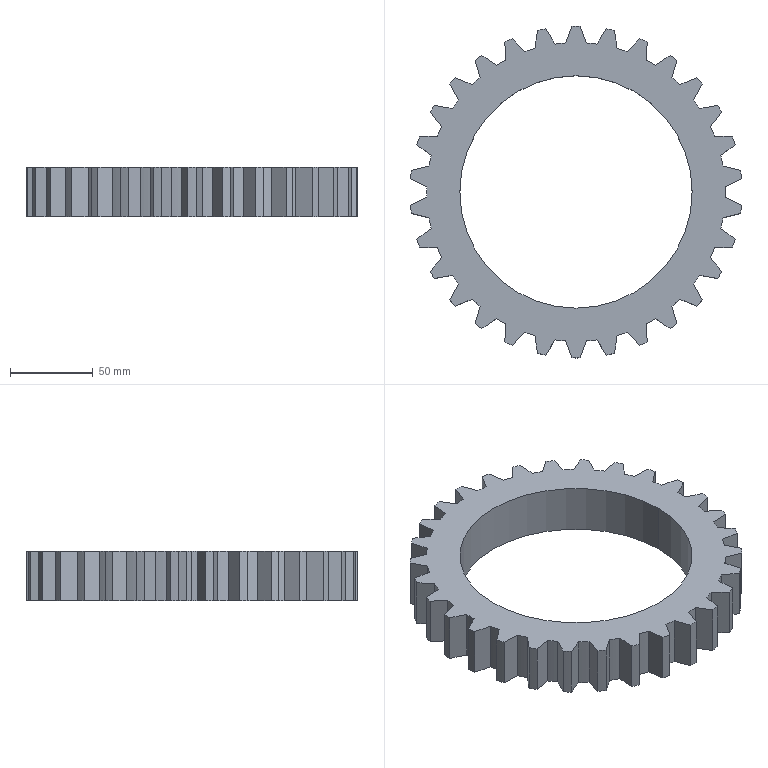Part | SolidWorks | features Extrusion 1 | 1 solid | 125 faces | box 199.365 x 200 x 30 mm | volume 379825 mm3 | cylinder 63 | plane 62 | commonest cylinder face diameters 180 x31 200 x30 140 x2